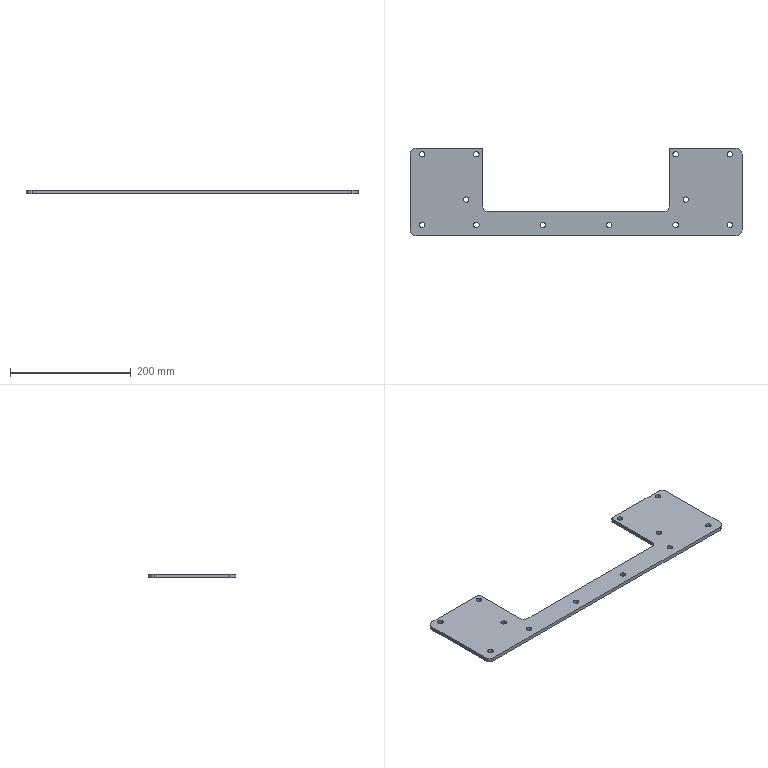Part | SolidWorks | features Fillet 4, HoleWzd 3, MirrorPattern 2, EdgeFlange 1, FlatPattern 1, ICE 1, SMBaseFlange 1, SheetMetal 1 | 1 solid | 42 faces | box 550 x 145 x 6 mm | volume 278339 mm3 | cylinder 32 | plane 10 | commonest cylinder face diameters 9 x24 20 x6 6 x2
STEP:
#1=CARTESIAN_POINT('',(160.5,62.5,0.));
#2=VERTEX_POINT('',#1);
#3=CARTESIAN_POINT('',(169.5,62.5,0.));
#4=VERTEX_POINT('',#3);
#5=CARTESIAN_POINT('',(165.,62.5,0.));
#6=DIRECTION('',(0.,0.,1.));
#7=DIRECTION('',(1.,0.,0.));
#8=AXIS2_PLACEMENT_3D('',#5,#6,#7);
#9=CIRCLE('',#8,4.5);
#10=EDGE_CURVE('',#2,#4,#9,.T.);
#11=ORIENTED_EDGE('',*,*,#10,.T.);
#12=CARTESIAN_POINT('',(169.5,62.5,-6.));
#13=VERTEX_POINT('',#12);
#14=CARTESIAN_POINT('',(169.5,62.5,-6.));
#15=DIRECTION('',(0.,0.,-1.));
#16=VECTOR('',#15,1000.);
#17=LINE('',#14,#16);
#18=EDGE_CURVE('',#4,#13,#17,.T.);
#19=ORIENTED_EDGE('',*,*,#18,.T.);
#20=CARTESIAN_POINT('',(160.5,62.5,-6.));
#21=VERTEX_POINT('',#20);
#22=CARTESIAN_POINT('',(165.,62.5,-6.));
#23=DIRECTION('',(0.,0.,-1.));
#24=DIRECTION('',(-1.,0.,0.));
#25=AXIS2_PLACEMENT_3D('',#22,#23,#24);
#26=CIRCLE('',#25,4.5);
#27=EDGE_CURVE('',#13,#21,#26,.T.);
#28=ORIENTED_EDGE('',*,*,#27,.T.);
#29=CARTESIAN_POINT('',(160.5,62.5,-6.));
#30=DIRECTION('',(0.,0.,-1.));
#31=VECTOR('',#30,1000.);
#32=LINE('',#29,#31);
#33=EDGE_CURVE('',#2,#21,#32,.T.);
#34=ORIENTED_EDGE('',*,*,#33,.F.);
#35=EDGE_LOOP('',(#11,#19,#28,#34));
#36=FACE_OUTER_BOUND('',#35,.T.);
#37=CARTESIAN_POINT('',(165.,62.5,-6.));
#38=DIRECTION('',(0.,0.,-1.));
#39=DIRECTION('',(-1.,0.,0.));
#40=AXIS2_PLACEMENT_3D('',#37,#38,#39);
#41=CYLINDRICAL_SURFACE('',#40,4.5);
#42=ADVANCED_FACE('',(#36),#41,.F.);
#43=CARTESIAN_POINT('',(50.5,-55.,0.));
#44=VERTEX_POINT('',#43);
#45=CARTESIAN_POINT('',(59.5,-55.,0.));
#46=VERTEX_POINT('',#45);
#47=CARTESIAN_POINT('',(55.,-55.,0.));
#48=DIRECTION('',(0.,0.,1.));
#49=DIRECTION('',(1.,0.,0.));
#50=AXIS2_PLACEMENT_3D('',#47,#48,#49);
#51=CIRCLE('',#50,4.5);
#52=EDGE_CURVE('',#44,#46,#51,.T.);
#53=ORIENTED_EDGE('',*,*,#52,.T.);
#54=CARTESIAN_POINT('',(59.5,-55.,-6.));
#55=VERTEX_POINT('',#54);
#56=CARTESIAN_POINT('',(59.5,-55.,-6.));
#57=DIRECTION('',(0.,0.,-1.));
#58=VECTOR('',#57,1000.);
#59=LINE('',#56,#58);
#60=EDGE_CURVE('',#46,#55,#59,.T.);
#61=ORIENTED_EDGE('',*,*,#60,.T.);
#62=CARTESIAN_POINT('',(50.5,-55.,-6.));
#63=VERTEX_POINT('',#62);
#64=CARTESIAN_POINT('',(55.,-55.,-6.));
#65=DIRECTION('',(0.,0.,-1.));
#66=DIRECTION('',(-1.,0.,0.));
#67=AXIS2_PLACEMENT_3D('',#64,#65,#66);
#68=CIRCLE('',#67,4.5);
#69=EDGE_CURVE('',#55,#63,#68,.T.);
#70=ORIENTED_EDGE('',*,*,#69,.T.);
#71=CARTESIAN_POINT('',(50.5,-55.,-6.));
#72=DIRECTION('',(0.,0.,-1.));
#73=VECTOR('',#72,1000.);
#74=LINE('',#71,#73);
#75=EDGE_CURVE('',#44,#63,#74,.T.);
#76=ORIENTED_EDGE('',*,*,#75,.F.);
#77=EDGE_LOOP('',(#53,#61,#70,#76));
#78=FACE_OUTER_BOUND('',#77,.T.);
#79=CARTESIAN_POINT('',(55.,-55.,-6.));
#80=DIRECTION('',(0.,0.,-1.));
#81=DIRECTION('',(-1.,0.,0.));
#82=AXIS2_PLACEMENT_3D('',#79,#80,#81);
#83=CYLINDRICAL_SURFACE('',#82,4.5);
#84=ADVANCED_FACE('',(#78),#83,.F.);
#85=CARTESIAN_POINT('',(-59.5,-55.,0.));
#86=VERTEX_POINT('',#85);
#87=CARTESIAN_POINT('',(-50.5,-55.,0.));
#88=VERTEX_POINT('',#87);
#89=CARTESIAN_POINT('',(-55.,-55.,0.));
#90=DIRECTION('',(0.,0.,1.));
#91=DIRECTION('',(1.,0.,0.));
#92=AXIS2_PLACEMENT_3D('',#89,#90,#91);
#93=CIRCLE('',#92,4.5);
#94=EDGE_CURVE('',#86,#88,#93,.T.);
#95=ORIENTED_EDGE('',*,*,#94,.T.);
#96=CARTESIAN_POINT('',(-50.5,-55.,-6.));
#97=VERTEX_POINT('',#96);
#98=CARTESIAN_POINT('',(-50.5,-55.,-6.));
#99=DIRECTION('',(0.,0.,-1.));
#100=VECTOR('',#99,1000.);
#101=LINE('',#98,#100);
#102=EDGE_CURVE('',#88,#97,#101,.T.);
#103=ORIENTED_EDGE('',*,*,#102,.T.);
#104=CARTESIAN_POINT('',(-59.5,-55.,-6.));
#105=VERTEX_POINT('',#104);
#106=CARTESIAN_POINT('',(-55.,-55.,-6.));
#107=DIRECTION('',(0.,0.,-1.));
#108=DIRECTION('',(-1.,0.,0.));
#109=AXIS2_PLACEMENT_3D('',#106,#107,#108);
#110=CIRCLE('',#109,4.5);
#111=EDGE_CURVE('',#97,#105,#110,.T.);
#112=ORIENTED_EDGE('',*,*,#111,.T.);
#113=CARTESIAN_POINT('',(-59.5,-55.,-6.));
#114=DIRECTION('',(0.,0.,-1.));
#115=VECTOR('',#114,1000.);
#116=LINE('',#113,#115);
#117=EDGE_CURVE('',#86,#105,#116,.T.);
#118=ORIENTED_EDGE('',*,*,#117,.F.);
#119=EDGE_LOOP('',(#95,#103,#112,#118));
#120=FACE_OUTER_BOUND('',#119,.T.);
#121=CARTESIAN_POINT('',(-55.,-55.,-6.));
#122=DIRECTION('',(0.,0.,-1.));
#123=DIRECTION('',(-1.,0.,0.));
#124=AXIS2_PLACEMENT_3D('',#121,#122,#123);
#125=CYLINDRICAL_SURFACE('',#124,4.5);
#126=ADVANCED_FACE('',(#120),#125,.F.);
#127=CARTESIAN_POINT('',(-169.5,-55.,0.));
#128=VERTEX_POINT('',#127);
#129=CARTESIAN_POINT('',(-160.5,-55.,0.));
#130=VERTEX_POINT('',#129);
#131=CARTESIAN_POINT('',(-165.,-55.,0.));
#132=DIRECTION('',(0.,0.,1.));
#133=DIRECTION('',(1.,0.,0.));
#134=AXIS2_PLACEMENT_3D('',#131,#132,#133);
#135=CIRCLE('',#134,4.5);
#136=EDGE_CURVE('',#128,#130,#135,.T.);
#137=ORIENTED_EDGE('',*,*,#136,.T.);
#138=CARTESIAN_POINT('',(-160.5,-55.,-6.));
#139=VERTEX_POINT('',#138);
#140=CARTESIAN_POINT('',(-160.5,-55.,-6.));
#141=DIRECTION('',(0.,0.,-1.));
#142=VECTOR('',#141,1000.);
#143=LINE('',#140,#142);
#144=EDGE_CURVE('',#130,#139,#143,.T.);
#145=ORIENTED_EDGE('',*,*,#144,.T.);
#146=CARTESIAN_POINT('',(-169.5,-55.,-6.));
#147=VERTEX_POINT('',#146);
#148=CARTESIAN_POINT('',(-165.,-55.,-6.));
#149=DIRECTION('',(0.,0.,-1.));
#150=DIRECTION('',(-1.,0.,0.));
#151=AXIS2_PLACEMENT_3D('',#148,#149,#150);
#152=CIRCLE('',#151,4.5);
#153=EDGE_CURVE('',#139,#147,#152,.T.);
#154=ORIENTED_EDGE('',*,*,#153,.T.);
#155=CARTESIAN_POINT('',(-169.5,-55.,-6.));
#156=DIRECTION('',(0.,0.,-1.));
#157=VECTOR('',#156,1000.);
#158=LINE('',#155,#157);
#159=EDGE_CURVE('',#128,#147,#158,.T.);
#160=ORIENTED_EDGE('',*,*,#159,.F.);
#161=EDGE_LOOP('',(#137,#145,#154,#160));
#162=FACE_OUTER_BOUND('',#161,.T.);
#163=CARTESIAN_POINT('',(-165.,-55.,-6.));
#164=DIRECTION('',(0.,0.,-1.));
#165=DIRECTION('',(-1.,0.,0.));
#166=AXIS2_PLACEMENT_3D('',#163,#164,#165);
#167=CYLINDRICAL_SURFACE('',#166,4.5);
#168=ADVANCED_FACE('',(#162),#167,.F.);
#169=CARTESIAN_POINT('',(-169.5,62.5,0.));
#170=VERTEX_POINT('',#169);
#171=CARTESIAN_POINT('',(-160.5,62.5,0.));
#172=VERTEX_POINT('',#171);
#173=CARTESIAN_POINT('',(-165.,62.5,0.));
#174=DIRECTION('',(0.,0.,1.));
#175=DIRECTION('',(1.,0.,0.));
#176=AXIS2_PLACEMENT_3D('',#173,#174,#175);
#177=CIRCLE('',#176,4.5);
#178=EDGE_CURVE('',#170,#172,#177,.T.);
#179=ORIENTED_EDGE('',*,*,#178,.T.);
#180=CARTESIAN_POINT('',(-160.5,62.5,-6.));
#181=VERTEX_POINT('',#180);
#182=CARTESIAN_POINT('',(-160.5,62.5,-6.));
#183=DIRECTION('',(0.,0.,-1.));
#184=VECTOR('',#183,1000.);
#185=LINE('',#182,#184);
#186=EDGE_CURVE('',#172,#181,#185,.T.);
#187=ORIENTED_EDGE('',*,*,#186,.T.);
#188=CARTESIAN_POINT('',(-169.5,62.5,-6.));
#189=VERTEX_POINT('',#188);
#190=CARTESIAN_POINT('',(-165.,62.5,-6.));
#191=DIRECTION('',(0.,0.,-1.));
#192=DIRECTION('',(-1.,0.,0.));
#193=AXIS2_PLACEMENT_3D('',#190,#191,#192);
#194=CIRCLE('',#193,4.5);
#195=EDGE_CURVE('',#181,#189,#194,.T.);
#196=ORIENTED_EDGE('',*,*,#195,.T.);
#197=CARTESIAN_POINT('',(-169.5,62.5,-6.));
#198=DIRECTION('',(0.,0.,-1.));
#199=VECTOR('',#198,1000.);
#200=LINE('',#197,#199);
#201=EDGE_CURVE('',#170,#189,#200,.T.);
#202=ORIENTED_EDGE('',*,*,#201,.F.);
#203=EDGE_LOOP('',(#179,#187,#196,#202));
#204=FACE_OUTER_BOUND('',#203,.T.);
#205=CARTESIAN_POINT('',(-165.,62.5,-6.));
#206=DIRECTION('',(0.,0.,-1.));
#207=DIRECTION('',(-1.,0.,0.));
#208=AXIS2_PLACEMENT_3D('',#205,#206,#207);
#209=CYLINDRICAL_SURFACE('',#208,4.5);
#210=ADVANCED_FACE('',(#204),#209,.F.);
#211=CARTESIAN_POINT('',(160.5,-55.,0.));
#212=VERTEX_POINT('',#211);
#213=CARTESIAN_POINT('',(169.5,-55.,0.));
#214=VERTEX_POINT('',#213);
#215=CARTESIAN_POINT('',(165.,-55.,0.));
#216=DIRECTION('',(0.,0.,1.));
#217=DIRECTION('',(1.,0.,0.));
#218=AXIS2_PLACEMENT_3D('',#215,#216,#217);
#219=CIRCLE('',#218,4.5);
#220=EDGE_CURVE('',#212,#214,#219,.T.);
#221=ORIENTED_EDGE('',*,*,#220,.T.);
#222=CARTESIAN_POINT('',(169.5,-55.,-6.));
#223=VERTEX_POINT('',#222);
#224=CARTESIAN_POINT('',(169.5,-55.,-6.));
#225=DIRECTION('',(0.,0.,-1.));
#226=VECTOR('',#225,1000.);
#227=LINE('',#224,#226);
#228=EDGE_CURVE('',#214,#223,#227,.T.);
#229=ORIENTED_EDGE('',*,*,#228,.T.);
#230=CARTESIAN_POINT('',(160.5,-55.,-6.));
#231=VERTEX_POINT('',#230);
#232=CARTESIAN_POINT('',(165.,-55.,-6.));
#233=DIRECTION('',(0.,0.,-1.));
#234=DIRECTION('',(-1.,0.,0.));
#235=AXIS2_PLACEMENT_3D('',#232,#233,#234);
#236=CIRCLE('',#235,4.5);
#237=EDGE_CURVE('',#223,#231,#236,.T.);
#238=ORIENTED_EDGE('',*,*,#237,.T.);
#239=CARTESIAN_POINT('',(160.5,-55.,-6.));
#240=DIRECTION('',(0.,0.,-1.));
#241=VECTOR('',#240,1000.);
#242=LINE('',#239,#241);
#243=EDGE_CURVE('',#212,#231,#242,.T.);
#244=ORIENTED_EDGE('',*,*,#243,.F.);
#245=EDGE_LOOP('',(#221,#229,#238,#244));
#246=FACE_OUTER_BOUND('',#245,.T.);
#247=CARTESIAN_POINT('',(165.,-55.,-6.));
#248=DIRECTION('',(0.,0.,-1.));
#249=DIRECTION('',(-1.,0.,0.));
#250=AXIS2_PLACEMENT_3D('',#247,#248,#249);
#251=CYLINDRICAL_SURFACE('',#250,4.5);
#252=ADVANCED_FACE('',(#246),#251,.F.);
#253=CARTESIAN_POINT('',(-259.5,-55.,0.));
#254=VERTEX_POINT('',#253);
#255=CARTESIAN_POINT('',(-250.5,-55.,0.));
#256=VERTEX_POINT('',#255);
#257=CARTESIAN_POINT('',(-255.,-55.,0.));
#258=DIRECTION('',(0.,0.,1.));
#259=DIRECTION('',(1.,0.,0.));
#260=AXIS2_PLACEMENT_3D('',#257,#258,#259);
#261=CIRCLE('',#260,4.5);
#262=EDGE_CURVE('',#254,#256,#261,.T.);
#263=ORIENTED_EDGE('',*,*,#262,.T.);
#264=CARTESIAN_POINT('',(-250.5,-55.,-6.));
#265=VERTEX_POINT('',#264);
#266=CARTESIAN_POINT('',(-250.5,-55.,-6.));
#267=DIRECTION('',(0.,0.,-1.));
#268=VECTOR('',#267,1000.);
#269=LINE('',#266,#268);
#270=EDGE_CURVE('',#256,#265,#269,.T.);
#271=ORIENTED_EDGE('',*,*,#270,.T.);
#272=CARTESIAN_POINT('',(-259.5,-55.,-6.));
#273=VERTEX_POINT('',#272);
#274=CARTESIAN_POINT('',(-255.,-55.,-6.));
#275=DIRECTION('',(0.,0.,-1.));
#276=DIRECTION('',(-1.,0.,0.));
#277=AXIS2_PLACEMENT_3D('',#274,#275,#276);
#278=CIRCLE('',#277,4.5);
#279=EDGE_CURVE('',#265,#273,#278,.T.);
#280=ORIENTED_EDGE('',*,*,#279,.T.);
#281=CARTESIAN_POINT('',(-259.5,-55.,-6.));
#282=DIRECTION('',(0.,0.,-1.));
#283=VECTOR('',#282,1000.);
#284=LINE('',#281,#283);
#285=EDGE_CURVE('',#254,#273,#284,.T.);
#286=ORIENTED_EDGE('',*,*,#285,.F.);
#287=EDGE_LOOP('',(#263,#271,#280,#286));
#288=FACE_OUTER_BOUND('',#287,.T.);
#289=CARTESIAN_POINT('',(-255.,-55.,-6.));
#290=DIRECTION('',(0.,0.,-1.));
#291=DIRECTION('',(-1.,0.,0.));
#292=AXIS2_PLACEMENT_3D('',#289,#290,#291);
#293=CYLINDRICAL_SURFACE('',#292,4.5);
#294=ADVANCED_FACE('',(#288),#293,.F.);
#295=CARTESIAN_POINT('',(250.5,-55.,0.));
#296=VERTEX_POINT('',#295);
#297=CARTESIAN_POINT('',(259.5,-55.,0.));
#298=VERTEX_POINT('',#297);
#299=CARTESIAN_POINT('',(255.,-55.,0.));
#300=DIRECTION('',(0.,0.,1.));
#301=DIRECTION('',(1.,0.,0.));
#302=AXIS2_PLACEMENT_3D('',#299,#300,#301);
#303=CIRCLE('',#302,4.5);
#304=EDGE_CURVE('',#296,#298,#303,.T.);
#305=ORIENTED_EDGE('',*,*,#304,.T.);
#306=CARTESIAN_POINT('',(259.5,-55.,-6.));
#307=VERTEX_POINT('',#306);
#308=CARTESIAN_POINT('',(259.5,-55.,-6.));
#309=DIRECTION('',(0.,0.,-1.));
#310=VECTOR('',#309,1000.);
#311=LINE('',#308,#310);
#312=EDGE_CURVE('',#298,#307,#311,.T.);
#313=ORIENTED_EDGE('',*,*,#312,.T.);
#314=CARTESIAN_POINT('',(250.5,-55.,-6.));
#315=VERTEX_POINT('',#314);
#316=CARTESIAN_POINT('',(255.,-55.,-6.));
#317=DIRECTION('',(0.,0.,-1.));
#318=DIRECTION('',(-1.,0.,0.));
#319=AXIS2_PLACEMENT_3D('',#316,#317,#318);
#320=CIRCLE('',#319,4.5);
#321=EDGE_CURVE('',#307,#315,#320,.T.);
#322=ORIENTED_EDGE('',*,*,#321,.T.);
#323=CARTESIAN_POINT('',(250.5,-55.,-6.));
#324=DIRECTION('',(0.,0.,-1.));
#325=VECTOR('',#324,1000.);
#326=LINE('',#323,#325);
#327=EDGE_CURVE('',#296,#315,#326,.T.);
#328=ORIENTED_EDGE('',*,*,#327,.F.);
#329=EDGE_LOOP('',(#305,#313,#322,#328));
#330=FACE_OUTER_BOUND('',#329,.T.);
#331=CARTESIAN_POINT('',(255.,-55.,-6.));
#332=DIRECTION('',(0.,0.,-1.));
#333=DIRECTION('',(-1.,0.,0.));
#334=AXIS2_PLACEMENT_3D('',#331,#332,#333);
#335=CYLINDRICAL_SURFACE('',#334,4.5);
#336=ADVANCED_FACE('',(#330),#335,.F.);
#337=CARTESIAN_POINT('',(250.5,62.5,0.));
#338=VERTEX_POINT('',#337);
#339=CARTESIAN_POINT('',(259.5,62.5,0.));
#340=VERTEX_POINT('',#339);
#341=CARTESIAN_POINT('',(255.,62.5,0.));
#342=DIRECTION('',(0.,0.,1.));
#343=DIRECTION('',(1.,0.,0.));
#344=AXIS2_PLACEMENT_3D('',#341,#342,#343);
#345=CIRCLE('',#344,4.5);
#346=EDGE_CURVE('',#338,#340,#345,.T.);
#347=ORIENTED_EDGE('',*,*,#346,.T.);
#348=CARTESIAN_POINT('',(259.5,62.5,-6.));
#349=VERTEX_POINT('',#348);
#350=CARTESIAN_POINT('',(259.5,62.5,-6.));
#351=DIRECTION('',(0.,0.,-1.));
#352=VECTOR('',#351,1000.);
#353=LINE('',#350,#352);
#354=EDGE_CURVE('',#340,#349,#353,.T.);
#355=ORIENTED_EDGE('',*,*,#354,.T.);
#356=CARTESIAN_POINT('',(250.5,62.5,-6.));
#357=VERTEX_POINT('',#356);
#358=CARTESIAN_POINT('',(255.,62.5,-6.));
#359=DIRECTION('',(0.,0.,-1.));
#360=DIRECTION('',(-1.,0.,0.));
#361=AXIS2_PLACEMENT_3D('',#358,#359,#360);
#362=CIRCLE('',#361,4.5);
#363=EDGE_CURVE('',#349,#357,#362,.T.);
#364=ORIENTED_EDGE('',*,*,#363,.T.);
#365=CARTESIAN_POINT('',(250.5,62.5,-6.));
#366=DIRECTION('',(0.,0.,-1.));
#367=VECTOR('',#366,1000.);
#368=LINE('',#365,#367);
#369=EDGE_CURVE('',#338,#357,#368,.T.);
#370=ORIENTED_EDGE('',*,*,#369,.F.);
#371=EDGE_LOOP('',(#347,#355,#364,#370));
#372=FACE_OUTER_BOUND('',#371,.T.);
#373=CARTESIAN_POINT('',(255.,62.5,-6.));
#374=DIRECTION('',(0.,0.,-1.));
#375=DIRECTION('',(-1.,0.,0.));
#376=AXIS2_PLACEMENT_3D('',#373,#374,#375);
#377=CYLINDRICAL_SURFACE('',#376,4.5);
#378=ADVANCED_FACE('',(#372),#377,.F.);
#379=CARTESIAN_POINT('',(-259.5,62.5,0.));
#380=VERTEX_POINT('',#379);
#381=CARTESIAN_POINT('',(-250.5,62.5,0.));
#382=VERTEX_POINT('',#381);
#383=CARTESIAN_POINT('',(-255.,62.5,0.));
#384=DIRECTION('',(0.,0.,1.));
#385=DIRECTION('',(1.,0.,0.));
#386=AXIS2_PLACEMENT_3D('',#383,#384,#385);
#387=CIRCLE('',#386,4.5);
#388=EDGE_CURVE('',#380,#382,#387,.T.);
#389=ORIENTED_EDGE('',*,*,#388,.T.);
#390=CARTESIAN_POINT('',(-250.5,62.5,-6.));
#391=VERTEX_POINT('',#390);
#392=CARTESIAN_POINT('',(-250.5,62.5,-6.));
#393=DIRECTION('',(0.,0.,-1.));
#394=VECTOR('',#393,1000.);
#395=LINE('',#392,#394);
#396=EDGE_CURVE('',#382,#391,#395,.T.);
#397=ORIENTED_EDGE('',*,*,#396,.T.);
#398=CARTESIAN_POINT('',(-259.5,62.5,-6.));
#399=VERTEX_POINT('',#398);
#400=CARTESIAN_POINT('',(-255.,62.5,-6.));
#401=DIRECTION('',(0.,0.,-1.));
#402=DIRECTION('',(-1.,0.,0.));
#403=AXIS2_PLACEMENT_3D('',#400,#401,#402);
#404=CIRCLE('',#403,4.5);
#405=EDGE_CURVE('',#391,#399,#404,.T.);
#406=ORIENTED_EDGE('',*,*,#405,.T.);
#407=CARTESIAN_POINT('',(-259.5,62.5,-6.));
#408=DIRECTION('',(0.,0.,-1.));
#409=VECTOR('',#408,1000.);
#410=LINE('',#407,#409);
#411=EDGE_CURVE('',#380,#399,#410,.T.);
#412=ORIENTED_EDGE('',*,*,#411,.F.);
#413=EDGE_LOOP('',(#389,#397,#406,#412));
#414=FACE_OUTER_BOUND('',#413,.T.);
#415=CARTESIAN_POINT('',(-255.,62.5,-6.));
#416=DIRECTION('',(0.,0.,-1.));
#417=DIRECTION('',(-1.,0.,0.));
#418=AXIS2_PLACEMENT_3D('',#415,#416,#417);
#419=CYLINDRICAL_SURFACE('',#418,4.5);
#420=ADVANCED_FACE('',(#414),#419,.F.);
#421=CARTESIAN_POINT('',(177.5,-12.5,-6.));
#422=VERTEX_POINT('',#421);
#423=CARTESIAN_POINT('',(186.5,-12.5,-6.));
#424=VERTEX_POINT('',#423);
#425=CARTESIAN_POINT('',(182.,-12.5,-6.));
#426=DIRECTION('',(0.,0.,1.));
#427=DIRECTION('',(1.,0.,0.));
#428=AXIS2_PLACEMENT_3D('',#425,#426,#427);
#429=CIRCLE('',#428,4.5);
#430=EDGE_CURVE('',#422,#424,#429,.T.);
#431=ORIENTED_EDGE('',*,*,#430,.F.);
#432=CARTESIAN_POINT('',(177.5,-12.5,0.));
#433=VERTEX_POINT('',#432);
#434=CARTESIAN_POINT('',(177.5,-12.5,0.));
#435=DIRECTION('',(0.,0.,1.));
#436=VECTOR('',#435,1000.);
#437=LINE('',#434,#436);
#438=EDGE_CURVE('',#422,#433,#437,.T.);
#439=ORIENTED_EDGE('',*,*,#438,.T.);
#440=CARTESIAN_POINT('',(186.5,-12.5,0.));
#441=VERTEX_POINT('',#440);
#442=CARTESIAN_POINT('',(182.,-12.5,0.));
#443=DIRECTION('',(0.,0.,1.));
#444=DIRECTION('',(1.,0.,0.));
#445=AXIS2_PLACEMENT_3D('',#442,#443,#444);
#446=CIRCLE('',#445,4.5);
#447=EDGE_CURVE('',#433,#441,#446,.T.);
#448=ORIENTED_EDGE('',*,*,#447,.T.);
#449=CARTESIAN_POINT('',(186.5,-12.5,0.));
#450=DIRECTION('',(0.,0.,1.));
#451=VECTOR('',#450,1000.);
#452=LINE('',#449,#451);
#453=EDGE_CURVE('',#424,#441,#452,.T.);
#454=ORIENTED_EDGE('',*,*,#453,.F.);
#455=EDGE_LOOP('',(#431,#439,#448,#454));
#456=FACE_OUTER_BOUND('',#455,.T.);
#457=CARTESIAN_POINT('',(182.,-12.5,0.));
#458=DIRECTION('',(0.,0.,1.));
#459=DIRECTION('',(1.,0.,0.));
#460=AXIS2_PLACEMENT_3D('',#457,#458,#459);
#461=CYLINDRICAL_SURFACE('',#460,4.5);
#462=ADVANCED_FACE('',(#456),#461,.F.);
#463=CARTESIAN_POINT('',(-186.5,-12.5,-6.));
#464=VERTEX_POINT('',#463);
#465=CARTESIAN_POINT('',(-177.5,-12.5,-6.));
#466=VERTEX_POINT('',#465);
#467=CARTESIAN_POINT('',(-182.,-12.5,-6.));
#468=DIRECTION('',(0.,0.,1.));
#469=DIRECTION('',(1.,0.,0.));
#470=AXIS2_PLACEMENT_3D('',#467,#468,#469);
#471=CIRCLE('',#470,4.5);
#472=EDGE_CURVE('',#464,#466,#471,.T.);
#473=ORIENTED_EDGE('',*,*,#472,.F.);
#474=CARTESIAN_POINT('',(-186.5,-12.5,0.));
#475=VERTEX_POINT('',#474);
#476=CARTESIAN_POINT('',(-186.5,-12.5,0.));
#477=DIRECTION('',(0.,0.,1.));
#478=VECTOR('',#477,1000.);
#479=LINE('',#476,#478);
#480=EDGE_CURVE('',#464,#475,#479,.T.);
#481=ORIENTED_EDGE('',*,*,#480,.T.);
#482=CARTESIAN_POINT('',(-177.5,-12.5,0.));
#483=VERTEX_POINT('',#482);
#484=CARTESIAN_POINT('',(-182.,-12.5,0.));
#485=DIRECTION('',(0.,0.,1.));
#486=DIRECTION('',(1.,0.,0.));
#487=AXIS2_PLACEMENT_3D('',#484,#485,#486);
#488=CIRCLE('',#487,4.5);
#489=EDGE_CURVE('',#475,#483,#488,.T.);
#490=ORIENTED_EDGE('',*,*,#489,.T.);
#491=CARTESIAN_POINT('',(-177.5,-12.5,0.));
#492=DIRECTION('',(0.,0.,1.));
#493=VECTOR('',#492,1000.);
#494=LINE('',#491,#493);
#495=EDGE_CURVE('',#466,#483,#494,.T.);
#496=ORIENTED_EDGE('',*,*,#495,.F.);
#497=EDGE_LOOP('',(#473,#481,#490,#496));
#498=FACE_OUTER_BOUND('',#497,.T.);
#499=CARTESIAN_POINT('',(-182.,-12.5,0.));
#500=DIRECTION('',(0.,0.,1.));
#501=DIRECTION('',(1.,0.,0.));
#502=AXIS2_PLACEMENT_3D('',#499,#500,#501);
#503=CYLINDRICAL_SURFACE('',#502,4.5);
#504=ADVANCED_FACE('',(#498),#503,.F.);
#505=CARTESIAN_POINT('',(-165.,62.5,-6.));
#506=DIRECTION('',(0.,0.,-1.));
#507=DIRECTION('',(-1.,0.,0.));
#508=AXIS2_PLACEMENT_3D('',#505,#506,#507);
#509=CIRCLE('',#508,4.5);
#510=EDGE_CURVE('',#189,#181,#509,.T.);
#511=ORIENTED_EDGE('',*,*,#510,.F.);
#512=ORIENTED_EDGE('',*,*,#195,.F.);
#513=EDGE_LOOP('',(#511,#512));
#514=FACE_BOUND('',#513,.T.);
#515=CARTESIAN_POINT('',(165.,-55.,-6.));
#516=DIRECTION('',(0.,0.,-1.));
#517=DIRECTION('',(-1.,0.,0.));
#518=AXIS2_PLACEMENT_3D('',#515,#516,#517);
#519=CIRCLE('',#518,4.5);
#520=EDGE_CURVE('',#231,#223,#519,.T.);
#521=ORIENTED_EDGE('',*,*,#520,.F.);
#522=ORIENTED_EDGE('',*,*,#237,.F.);
#523=EDGE_LOOP('',(#521,#522));
#524=FACE_BOUND('',#523,.T.);
#525=CARTESIAN_POINT('',(-255.,-55.,-6.));
#526=DIRECTION('',(0.,0.,-1.));
#527=DIRECTION('',(-1.,0.,0.));
#528=AXIS2_PLACEMENT_3D('',#525,#526,#527);
#529=CIRCLE('',#528,4.5);
#530=EDGE_CURVE('',#273,#265,#529,.T.);
#531=ORIENTED_EDGE('',*,*,#530,.F.);
#532=ORIENTED_EDGE('',*,*,#279,.F.);
#533=EDGE_LOOP('',(#531,#532));
#534=FACE_BOUND('',#533,.T.);
#535=CARTESIAN_POINT('',(255.,-55.,-6.));
#536=DIRECTION('',(0.,0.,-1.));
#537=DIRECTION('',(-1.,0.,0.));
#538=AXIS2_PLACEMENT_3D('',#535,#536,#537);
#539=CIRCLE('',#538,4.5);
#540=EDGE_CURVE('',#315,#307,#539,.T.);
#541=ORIENTED_EDGE('',*,*,#540,.F.);
#542=ORIENTED_EDGE('',*,*,#321,.F.);
#543=EDGE_LOOP('',(#541,#542));
#544=FACE_BOUND('',#543,.T.);
#545=CARTESIAN_POINT('',(255.,62.5,-6.));
#546=DIRECTION('',(0.,0.,-1.));
#547=DIRECTION('',(-1.,0.,0.));
#548=AXIS2_PLACEMENT_3D('',#545,#546,#547);
#549=CIRCLE('',#548,4.5);
#550=EDGE_CURVE('',#357,#349,#549,.T.);
#551=ORIENTED_EDGE('',*,*,#550,.F.);
#552=ORIENTED_EDGE('',*,*,#363,.F.);
#553=EDGE_LOOP('',(#551,#552));
#554=FACE_BOUND('',#553,.T.);
#555=CARTESIAN_POINT('',(-255.,62.5,-6.));
#556=DIRECTION('',(0.,0.,-1.));
#557=DIRECTION('',(-1.,0.,0.));
#558=AXIS2_PLACEMENT_3D('',#555,#556,#557);
#559=CIRCLE('',#558,4.5);
#560=EDGE_CURVE('',#399,#391,#559,.T.);
#561=ORIENTED_EDGE('',*,*,#560,.F.);
#562=ORIENTED_EDGE('',*,*,#405,.F.);
#563=EDGE_LOOP('',(#561,#562));
#564=FACE_BOUND('',#563,.T.);
#565=CARTESIAN_POINT('',(182.,-12.5,-6.));
#566=DIRECTION('',(0.,0.,1.));
#567=DIRECTION('',(1.,0.,0.));
#568=AXIS2_PLACEMENT_3D('',#565,#566,#567);
#569=CIRCLE('',#568,4.5);
#570=EDGE_CURVE('',#424,#422,#569,.T.);
#571=ORIENTED_EDGE('',*,*,#570,.T.);
#572=ORIENTED_EDGE('',*,*,#430,.T.);
#573=EDGE_LOOP('',(#571,#572));
#574=FACE_BOUND('',#573,.T.);
#575=CARTESIAN_POINT('',(-182.,-12.5,-6.));
#576=DIRECTION('',(0.,0.,1.));
#577=DIRECTION('',(1.,0.,0.));
#578=AXIS2_PLACEMENT_3D('',#575,#576,#577);
#579=CIRCLE('',#578,4.5);
#580=EDGE_CURVE('',#466,#464,#579,.T.);
#581=ORIENTED_EDGE('',*,*,#580,.T.);
#582=ORIENTED_EDGE('',*,*,#472,.T.);
#583=EDGE_LOOP('',(#581,#582));
#584=FACE_BOUND('',#583,.T.);
#585=CARTESIAN_POINT('',(155.,-22.5,-6.));
#586=VERTEX_POINT('',#585);
#587=CARTESIAN_POINT('',(155.,69.5,-6.));
#588=VERTEX_POINT('',#587);
#589=CARTESIAN_POINT('',(155.,72.5,-6.));
#590=DIRECTION('',(0.,1.,0.));
#591=VECTOR('',#590,1000.);
#592=LINE('',#589,#591);
#593=EDGE_CURVE('',#586,#588,#592,.T.);
#594=ORIENTED_EDGE('',*,*,#593,.T.);
#595=CARTESIAN_POINT('',(158.,72.5,-6.));
#596=VERTEX_POINT('',#595);
#597=CARTESIAN_POINT('',(158.,69.5,-6.));
#598=DIRECTION('',(0.,0.,-1.));
#599=DIRECTION('',(1.,0.,0.));
#600=AXIS2_PLACEMENT_3D('',#597,#598,#599);
#601=CIRCLE('',#600,3.);
#602=EDGE_CURVE('',#588,#596,#601,.T.);
#603=ORIENTED_EDGE('',*,*,#602,.T.);
#604=CARTESIAN_POINT('',(265.,72.5,-6.));
#605=VERTEX_POINT('',#604);
#606=CARTESIAN_POINT('',(-275.,72.5,-6.));
#607=DIRECTION('',(-1.,0.,0.));
#608=VECTOR('',#607,1000.);
#609=LINE('',#606,#608);
#610=EDGE_CURVE('',#605,#596,#609,.T.);
#611=ORIENTED_EDGE('',*,*,#610,.F.);
#612=CARTESIAN_POINT('',(275.,62.5,-6.));
#613=VERTEX_POINT('',#612);
#614=CARTESIAN_POINT('',(265.,62.5,-6.));
#615=DIRECTION('',(0.,0.,-1.));
#616=DIRECTION('',(1.,0.,0.));
#617=AXIS2_PLACEMENT_3D('',#614,#615,#616);
#618=CIRCLE('',#617,10.);
#619=EDGE_CURVE('',#605,#613,#618,.T.);
#620=ORIENTED_EDGE('',*,*,#619,.T.);
#621=CARTESIAN_POINT('',(275.,-62.5,-6.));
#622=VERTEX_POINT('',#621);
#623=CARTESIAN_POINT('',(275.,72.5,-6.));
#624=DIRECTION('',(0.,1.,0.));
#625=VECTOR('',#624,1000.);
#626=LINE('',#623,#625);
#627=EDGE_CURVE('',#622,#613,#626,.T.);
#628=ORIENTED_EDGE('',*,*,#627,.F.);
#629=CARTESIAN_POINT('',(265.,-72.5,-6.));
#630=VERTEX_POINT('',#629);
#631=CARTESIAN_POINT('',(265.,-62.5,-6.));
#632=DIRECTION('',(0.,0.,-1.));
#633=DIRECTION('',(1.,0.,0.));
#634=AXIS2_PLACEMENT_3D('',#631,#632,#633);
#635=CIRCLE('',#634,10.);
#636=EDGE_CURVE('',#622,#630,#635,.T.);
#637=ORIENTED_EDGE('',*,*,#636,.T.);
#638=CARTESIAN_POINT('',(-265.,-72.5,-6.));
#639=VERTEX_POINT('',#638);
#640=CARTESIAN_POINT('',(-275.,-72.5,-6.));
#641=DIRECTION('',(1.,0.,0.));
#642=VECTOR('',#641,1000.);
#643=LINE('',#640,#642);
#644=EDGE_CURVE('',#639,#630,#643,.T.);
#645=ORIENTED_EDGE('',*,*,#644,.F.);
#646=CARTESIAN_POINT('',(-275.,-62.5,-6.));
#647=VERTEX_POINT('',#646);
#648=CARTESIAN_POINT('',(-265.,-62.5,-6.));
#649=DIRECTION('',(0.,0.,-1.));
#650=DIRECTION('',(1.,0.,0.));
#651=AXIS2_PLACEMENT_3D('',#648,#649,#650);
#652=CIRCLE('',#651,10.);
#653=EDGE_CURVE('',#639,#647,#652,.T.);
#654=ORIENTED_EDGE('',*,*,#653,.T.);
#655=CARTESIAN_POINT('',(-275.,62.5,-6.));
#656=VERTEX_POINT('',#655);
#657=CARTESIAN_POINT('',(-275.,72.5,-6.));
#658=DIRECTION('',(0.,-1.,0.));
#659=VECTOR('',#658,1000.);
#660=LINE('',#657,#659);
#661=EDGE_CURVE('',#656,#647,#660,.T.);
#662=ORIENTED_EDGE('',*,*,#661,.F.);
#663=CARTESIAN_POINT('',(-265.,72.5,-6.));
#664=VERTEX_POINT('',#663);
#665=CARTESIAN_POINT('',(-265.,62.5,-6.));
#666=DIRECTION('',(0.,0.,-1.));
#667=DIRECTION('',(1.,0.,0.));
#668=AXIS2_PLACEMENT_3D('',#665,#666,#667);
#669=CIRCLE('',#668,10.);
#670=EDGE_CURVE('',#656,#664,#669,.T.);
#671=ORIENTED_EDGE('',*,*,#670,.T.);
#672=CARTESIAN_POINT('',(-158.,72.5,-6.));
#673=VERTEX_POINT('',#672);
#674=CARTESIAN_POINT('',(-275.,72.5,-6.));
#675=DIRECTION('',(-1.,0.,0.));
#676=VECTOR('',#675,1000.);
#677=LINE('',#674,#676);
#678=EDGE_CURVE('',#673,#664,#677,.T.);
#679=ORIENTED_EDGE('',*,*,#678,.F.);
#680=CARTESIAN_POINT('',(-155.,69.5,-6.));
#681=VERTEX_POINT('',#680);
#682=CARTESIAN_POINT('',(-158.,69.5,-6.));
#683=DIRECTION('',(0.,0.,-1.));
#684=DIRECTION('',(1.,0.,0.));
#685=AXIS2_PLACEMENT_3D('',#682,#683,#684);
#686=CIRCLE('',#685,3.);
#687=EDGE_CURVE('',#673,#681,#686,.T.);
#688=ORIENTED_EDGE('',*,*,#687,.T.);
#689=CARTESIAN_POINT('',(-155.,-22.5,-6.));
#690=VERTEX_POINT('',#689);
#691=CARTESIAN_POINT('',(-155.,72.5,-6.));
#692=DIRECTION('',(0.,-1.,0.));
#693=VECTOR('',#692,1000.);
#694=LINE('',#691,#693);
#695=EDGE_CURVE('',#681,#690,#694,.T.);
#696=ORIENTED_EDGE('',*,*,#695,.T.);
#697=CARTESIAN_POINT('',(-145.,-32.5,-6.));
#698=VERTEX_POINT('',#697);
#699=CARTESIAN_POINT('',(-145.,-22.5,-6.));
#700=DIRECTION('',(0.,0.,1.));
#701=DIRECTION('',(1.,0.,0.));
#702=AXIS2_PLACEMENT_3D('',#699,#700,#701);
#703=CIRCLE('',#702,10.);
#704=EDGE_CURVE('',#690,#698,#703,.T.);
#705=ORIENTED_EDGE('',*,*,#704,.T.);
#706=CARTESIAN_POINT('',(145.,-32.5,-6.));
#707=VERTEX_POINT('',#706);
#708=CARTESIAN_POINT('',(-155.,-32.5,-6.));
#709=DIRECTION('',(1.,0.,0.));
#710=VECTOR('',#709,1000.);
#711=LINE('',#708,#710);
#712=EDGE_CURVE('',#698,#707,#711,.T.);
#713=ORIENTED_EDGE('',*,*,#712,.T.);
#714=CARTESIAN_POINT('',(145.,-22.5,-6.));
#715=DIRECTION('',(0.,0.,1.));
#716=DIRECTION('',(1.,0.,0.));
#717=AXIS2_PLACEMENT_3D('',#714,#715,#716);
#718=CIRCLE('',#717,10.);
#719=EDGE_CURVE('',#707,#586,#718,.T.);
#720=ORIENTED_EDGE('',*,*,#719,.T.);
#721=EDGE_LOOP('',(#594,#603,#611,#620,#628,#637,#645,#654,#662,#671,#679,#688,#696,#705,#713,#720));
#722=FACE_OUTER_BOUND('',#721,.T.);
#723=CARTESIAN_POINT('',(-165.,-55.,-6.));
#724=DIRECTION('',(0.,0.,-1.));
#725=DIRECTION('',(-1.,0.,0.));
#726=AXIS2_PLACEMENT_3D('',#723,#724,#725);
#727=CIRCLE('',#726,4.5);
#728=EDGE_CURVE('',#147,#139,#727,.T.);
#729=ORIENTED_EDGE('',*,*,#728,.F.);
#730=ORIENTED_EDGE('',*,*,#153,.F.);
#731=EDGE_LOOP('',(#729,#730));
#732=FACE_BOUND('',#731,.T.);
#733=CARTESIAN_POINT('',(-55.,-55.,-6.));
#734=DIRECTION('',(0.,0.,-1.));
#735=DIRECTION('',(-1.,0.,0.));
#736=AXIS2_PLACEMENT_3D('',#733,#734,#735);
#737=CIRCLE('',#736,4.5);
#738=EDGE_CURVE('',#105,#97,#737,.T.);
#739=ORIENTED_EDGE('',*,*,#738,.F.);
#740=ORIENTED_EDGE('',*,*,#111,.F.);
#741=EDGE_LOOP('',(#739,#740));
#742=FACE_BOUND('',#741,.T.);
#743=CARTESIAN_POINT('',(55.,-55.,-6.));
#744=DIRECTION('',(0.,0.,-1.));
#745=DIRECTION('',(-1.,0.,0.));
#746=AXIS2_PLACEMENT_3D('',#743,#744,#745);
#747=CIRCLE('',#746,4.5);
#748=EDGE_CURVE('',#63,#55,#747,.T.);
#749=ORIENTED_EDGE('',*,*,#748,.F.);
#750=ORIENTED_EDGE('',*,*,#69,.F.);
#751=EDGE_LOOP('',(#749,#750));
#752=FACE_BOUND('',#751,.T.);
#753=CARTESIAN_POINT('',(165.,62.5,-6.));
#754=DIRECTION('',(0.,0.,-1.));
#755=DIRECTION('',(-1.,0.,0.));
#756=AXIS2_PLACEMENT_3D('',#753,#754,#755);
#757=CIRCLE('',#756,4.5);
#758=EDGE_CURVE('',#21,#13,#757,.T.);
#759=ORIENTED_EDGE('',*,*,#758,.F.);
#760=ORIENTED_EDGE('',*,*,#27,.F.);
#761=EDGE_LOOP('',(#759,#760));
#762=FACE_BOUND('',#761,.T.);
#763=CARTESIAN_POINT('',(0.,0.,-6.));
#764=DIRECTION('',(0.,0.,1.));
#765=DIRECTION('',(1.,0.,0.));
#766=AXIS2_PLACEMENT_3D('',#763,#764,#765);
#767=PLANE('',#766);
#768=ADVANCED_FACE('',(#514,#524,#534,#544,#554,#564,#574,#584,#722,#732,#742,#752,#762),#767,.F.);
#769=CARTESIAN_POINT('',(-158.,72.5,0.));
#770=VERTEX_POINT('',#769);
#771=CARTESIAN_POINT('',(-265.,72.5,0.));
#772=VERTEX_POINT('',#771);
#773=CARTESIAN_POINT('',(-275.,72.5,0.));
#774=DIRECTION('',(-1.,0.,0.));
#775=VECTOR('',#774,1000.);
#776=LINE('',#773,#775);
#777=EDGE_CURVE('',#770,#772,#776,.T.);
#778=ORIENTED_EDGE('',*,*,#777,.F.);
#779=CARTESIAN_POINT('',(-158.,72.5,-6.));
#780=DIRECTION('',(0.,0.,-1.));
#781=VECTOR('',#780,1000.);
#782=LINE('',#779,#781);
#783=EDGE_CURVE('',#770,#673,#782,.T.);
#784=ORIENTED_EDGE('',*,*,#783,.T.);
#785=ORIENTED_EDGE('',*,*,#678,.T.);
#786=CARTESIAN_POINT('',(-265.,72.5,-6.));
#787=DIRECTION('',(0.,0.,1.));
#788=VECTOR('',#787,1000.);
#789=LINE('',#786,#788);
#790=EDGE_CURVE('',#664,#772,#789,.T.);
#791=ORIENTED_EDGE('',*,*,#790,.T.);
#792=EDGE_LOOP('',(#778,#784,#785,#791));
#793=FACE_OUTER_BOUND('',#792,.T.);
#794=CARTESIAN_POINT('',(-275.,72.5,-6.));
#795=DIRECTION('',(0.,1.,0.));
#796=DIRECTION('',(0.,0.,1.));
#797=AXIS2_PLACEMENT_3D('',#794,#795,#796);
#798=PLANE('',#797);
#799=ADVANCED_FACE('',(#793),#798,.T.);
#800=ORIENTED_EDGE('',*,*,#661,.T.);
#801=CARTESIAN_POINT('',(-275.,-62.5,0.));
#802=VERTEX_POINT('',#801);
#803=CARTESIAN_POINT('',(-275.,-62.5,-6.));
#804=DIRECTION('',(0.,0.,1.));
#805=VECTOR('',#804,1000.);
#806=LINE('',#803,#805);
#807=EDGE_CURVE('',#647,#802,#806,.T.);
#808=ORIENTED_EDGE('',*,*,#807,.T.);
#809=CARTESIAN_POINT('',(-275.,62.5,0.));
#810=VERTEX_POINT('',#809);
#811=CARTESIAN_POINT('',(-275.,72.5,0.));
#812=DIRECTION('',(0.,-1.,0.));
#813=VECTOR('',#812,1000.);
#814=LINE('',#811,#813);
#815=EDGE_CURVE('',#810,#802,#814,.T.);
#816=ORIENTED_EDGE('',*,*,#815,.F.);
#817=CARTESIAN_POINT('',(-275.,62.5,-6.));
#818=DIRECTION('',(0.,0.,-1.));
#819=VECTOR('',#818,1000.);
#820=LINE('',#817,#819);
#821=EDGE_CURVE('',#810,#656,#820,.T.);
#822=ORIENTED_EDGE('',*,*,#821,.T.);
#823=EDGE_LOOP('',(#800,#808,#816,#822));
#824=FACE_OUTER_BOUND('',#823,.T.);
#825=CARTESIAN_POINT('',(-275.,72.5,-6.));
#826=DIRECTION('',(-1.,0.,0.));
#827=DIRECTION('',(0.,0.,1.));
#828=AXIS2_PLACEMENT_3D('',#825,#826,#827);
#829=PLANE('',#828);
#830=ADVANCED_FACE('',(#824),#829,.T.);
#831=ORIENTED_EDGE('',*,*,#610,.T.);
#832=CARTESIAN_POINT('',(158.,72.5,0.));
#833=VERTEX_POINT('',#832);
#834=CARTESIAN_POINT('',(158.,72.5,0.));
#835=DIRECTION('',(0.,0.,1.));
#836=VECTOR('',#835,1000.);
#837=LINE('',#834,#836);
#838=EDGE_CURVE('',#596,#833,#837,.T.);
#839=ORIENTED_EDGE('',*,*,#838,.T.);
#840=CARTESIAN_POINT('',(265.,72.5,0.));
#841=VERTEX_POINT('',#840);
#842=CARTESIAN_POINT('',(-275.,72.5,0.));
#843=DIRECTION('',(-1.,0.,0.));
#844=VECTOR('',#843,1000.);
#845=LINE('',#842,#844);
#846=EDGE_CURVE('',#841,#833,#845,.T.);
#847=ORIENTED_EDGE('',*,*,#846,.F.);
#848=CARTESIAN_POINT('',(265.,72.5,-6.));
#849=DIRECTION('',(0.,0.,-1.));
#850=VECTOR('',#849,1000.);
#851=LINE('',#848,#850);
#852=EDGE_CURVE('',#841,#605,#851,.T.);
#853=ORIENTED_EDGE('',*,*,#852,.T.);
#854=EDGE_LOOP('',(#831,#839,#847,#853));
#855=FACE_OUTER_BOUND('',#854,.T.);
#856=CARTESIAN_POINT('',(-275.,72.5,-6.));
#857=DIRECTION('',(0.,1.,0.));
#858=DIRECTION('',(0.,0.,1.));
#859=AXIS2_PLACEMENT_3D('',#856,#857,#858);
#860=PLANE('',#859);
#861=ADVANCED_FACE('',(#855),#860,.T.);
#862=CARTESIAN_POINT('',(275.,-62.5,0.));
#863=VERTEX_POINT('',#862);
#864=CARTESIAN_POINT('',(275.,62.5,0.));
#865=VERTEX_POINT('',#864);
#866=CARTESIAN_POINT('',(275.,72.5,0.));
#867=DIRECTION('',(0.,1.,0.));
#868=VECTOR('',#867,1000.);
#869=LINE('',#866,#868);
#870=EDGE_CURVE('',#863,#865,#869,.T.);
#871=ORIENTED_EDGE('',*,*,#870,.F.);
#872=CARTESIAN_POINT('',(275.,-62.5,-6.));
#873=DIRECTION('',(0.,0.,-1.));
#874=VECTOR('',#873,1000.);
#875=LINE('',#872,#874);
#876=EDGE_CURVE('',#863,#622,#875,.T.);
#877=ORIENTED_EDGE('',*,*,#876,.T.);
#878=ORIENTED_EDGE('',*,*,#627,.T.);
#879=CARTESIAN_POINT('',(275.,62.5,-6.));
#880=DIRECTION('',(0.,0.,1.));
#881=VECTOR('',#880,1000.);
#882=LINE('',#879,#881);
#883=EDGE_CURVE('',#613,#865,#882,.T.);
#884=ORIENTED_EDGE('',*,*,#883,.T.);
#885=EDGE_LOOP('',(#871,#877,#878,#884));
#886=FACE_OUTER_BOUND('',#885,.T.);
#887=CARTESIAN_POINT('',(275.,72.5,-6.));
#888=DIRECTION('',(1.,0.,0.));
#889=DIRECTION('',(0.,0.,-1.));
#890=AXIS2_PLACEMENT_3D('',#887,#888,#889);
#891=PLANE('',#890);
#892=ADVANCED_FACE('',(#886),#891,.T.);
#893=ORIENTED_EDGE('',*,*,#644,.T.);
#894=CARTESIAN_POINT('',(265.,-72.5,0.));
#895=VERTEX_POINT('',#894);
#896=CARTESIAN_POINT('',(265.,-72.5,-6.));
#897=DIRECTION('',(0.,0.,1.));
#898=VECTOR('',#897,1000.);
#899=LINE('',#896,#898);
#900=EDGE_CURVE('',#630,#895,#899,.T.);
#901=ORIENTED_EDGE('',*,*,#900,.T.);
#902=CARTESIAN_POINT('',(-265.,-72.5,0.));
#903=VERTEX_POINT('',#902);
#904=CARTESIAN_POINT('',(-275.,-72.5,0.));
#905=DIRECTION('',(1.,0.,0.));
#906=VECTOR('',#905,1000.);
#907=LINE('',#904,#906);
#908=EDGE_CURVE('',#903,#895,#907,.T.);
#909=ORIENTED_EDGE('',*,*,#908,.F.);
#910=CARTESIAN_POINT('',(-265.,-72.5,-6.));
#911=DIRECTION('',(0.,0.,-1.));
#912=VECTOR('',#911,1000.);
#913=LINE('',#910,#912);
#914=EDGE_CURVE('',#903,#639,#913,.T.);
#915=ORIENTED_EDGE('',*,*,#914,.T.);
#916=EDGE_LOOP('',(#893,#901,#909,#915));
#917=FACE_OUTER_BOUND('',#916,.T.);
#918=CARTESIAN_POINT('',(-275.,-72.5,-6.));
#919=DIRECTION('',(0.,-1.,0.));
#920=DIRECTION('',(0.,0.,-1.));
#921=AXIS2_PLACEMENT_3D('',#918,#919,#920);
#922=PLANE('',#921);
#923=ADVANCED_FACE('',(#917),#922,.T.);
#924=ORIENTED_EDGE('',*,*,#10,.F.);
#925=CARTESIAN_POINT('',(165.,62.5,0.));
#926=DIRECTION('',(0.,0.,1.));
#927=DIRECTION('',(1.,0.,0.));
#928=AXIS2_PLACEMENT_3D('',#925,#926,#927);
#929=CIRCLE('',#928,4.5);
#930=EDGE_CURVE('',#4,#2,#929,.T.);
#931=ORIENTED_EDGE('',*,*,#930,.F.);
#932=EDGE_LOOP('',(#924,#931));
#933=FACE_BOUND('',#932,.T.);
#934=ORIENTED_EDGE('',*,*,#52,.F.);
#935=CARTESIAN_POINT('',(55.,-55.,0.));
#936=DIRECTION('',(0.,0.,1.));
#937=DIRECTION('',(1.,0.,0.));
#938=AXIS2_PLACEMENT_3D('',#935,#936,#937);
#939=CIRCLE('',#938,4.5);
#940=EDGE_CURVE('',#46,#44,#939,.T.);
#941=ORIENTED_EDGE('',*,*,#940,.F.);
#942=EDGE_LOOP('',(#934,#941));
#943=FACE_BOUND('',#942,.T.);
#944=ORIENTED_EDGE('',*,*,#94,.F.);
#945=CARTESIAN_POINT('',(-55.,-55.,0.));
#946=DIRECTION('',(0.,0.,1.));
#947=DIRECTION('',(1.,0.,0.));
#948=AXIS2_PLACEMENT_3D('',#945,#946,#947);
#949=CIRCLE('',#948,4.5);
#950=EDGE_CURVE('',#88,#86,#949,.T.);
#951=ORIENTED_EDGE('',*,*,#950,.F.);
#952=EDGE_LOOP('',(#944,#951));
#953=FACE_BOUND('',#952,.T.);
#954=ORIENTED_EDGE('',*,*,#136,.F.);
#955=CARTESIAN_POINT('',(-165.,-55.,0.));
#956=DIRECTION('',(0.,0.,1.));
#957=DIRECTION('',(1.,0.,0.));
#958=AXIS2_PLACEMENT_3D('',#955,#956,#957);
#959=CIRCLE('',#958,4.5);
#960=EDGE_CURVE('',#130,#128,#959,.T.);
#961=ORIENTED_EDGE('',*,*,#960,.F.);
#962=EDGE_LOOP('',(#954,#961));
#963=FACE_BOUND('',#962,.T.);
#964=ORIENTED_EDGE('',*,*,#178,.F.);
#965=CARTESIAN_POINT('',(-165.,62.5,0.));
#966=DIRECTION('',(0.,0.,1.));
#967=DIRECTION('',(1.,0.,0.));
#968=AXIS2_PLACEMENT_3D('',#965,#966,#967);
#969=CIRCLE('',#968,4.5);
#970=EDGE_CURVE('',#172,#170,#969,.T.);
#971=ORIENTED_EDGE('',*,*,#970,.F.);
#972=EDGE_LOOP('',(#964,#971));
#973=FACE_BOUND('',#972,.T.);
#974=ORIENTED_EDGE('',*,*,#220,.F.);
#975=CARTESIAN_POINT('',(165.,-55.,0.));
#976=DIRECTION('',(0.,0.,1.));
#977=DIRECTION('',(1.,0.,0.));
#978=AXIS2_PLACEMENT_3D('',#975,#976,#977);
#979=CIRCLE('',#978,4.5);
#980=EDGE_CURVE('',#214,#212,#979,.T.);
#981=ORIENTED_EDGE('',*,*,#980,.F.);
#982=EDGE_LOOP('',(#974,#981));
#983=FACE_BOUND('',#982,.T.);
#984=ORIENTED_EDGE('',*,*,#262,.F.);
#985=CARTESIAN_POINT('',(-255.,-55.,0.));
#986=DIRECTION('',(0.,0.,1.));
#987=DIRECTION('',(1.,0.,0.));
#988=AXIS2_PLACEMENT_3D('',#985,#986,#987);
#989=CIRCLE('',#988,4.5);
#990=EDGE_CURVE('',#256,#254,#989,.T.);
#991=ORIENTED_EDGE('',*,*,#990,.F.);
#992=EDGE_LOOP('',(#984,#991));
#993=FACE_BOUND('',#992,.T.);
#994=ORIENTED_EDGE('',*,*,#304,.F.);
#995=CARTESIAN_POINT('',(255.,-55.,0.));
#996=DIRECTION('',(0.,0.,1.));
#997=DIRECTION('',(1.,0.,0.));
#998=AXIS2_PLACEMENT_3D('',#995,#996,#997);
#999=CIRCLE('',#998,4.5);
#1000=EDGE_CURVE('',#298,#296,#999,.T.);
#1001=ORIENTED_EDGE('',*,*,#1000,.F.);
#1002=EDGE_LOOP('',(#994,#1001));
#1003=FACE_BOUND('',#1002,.T.);
#1004=ORIENTED_EDGE('',*,*,#346,.F.);
#1005=CARTESIAN_POINT('',(255.,62.5,0.));
#1006=DIRECTION('',(0.,0.,1.));
#1007=DIRECTION('',(1.,0.,0.));
#1008=AXIS2_PLACEMENT_3D('',#1005,#1006,#1007);
#1009=CIRCLE('',#1008,4.5);
#1010=EDGE_CURVE('',#340,#338,#1009,.T.);
#1011=ORIENTED_EDGE('',*,*,#1010,.F.);
#1012=EDGE_LOOP('',(#1004,#1011));
#1013=FACE_BOUND('',#1012,.T.);
#1014=ORIENTED_EDGE('',*,*,#388,.F.);
#1015=CARTESIAN_POINT('',(-255.,62.5,0.));
#1016=DIRECTION('',(0.,0.,1.));
#1017=DIRECTION('',(1.,0.,0.));
#1018=AXIS2_PLACEMENT_3D('',#1015,#1016,#1017);
#1019=CIRCLE('',#1018,4.5);
#1020=EDGE_CURVE('',#382,#380,#1019,.T.);
#1021=ORIENTED_EDGE('',*,*,#1020,.F.);
#1022=EDGE_LOOP('',(#1014,#1021));
#1023=FACE_BOUND('',#1022,.T.);
#1024=CARTESIAN_POINT('',(182.,-12.5,0.));
#1025=DIRECTION('',(0.,0.,1.));
#1026=DIRECTION('',(1.,0.,0.));
#1027=AXIS2_PLACEMENT_3D('',#1024,#1025,#1026);
#1028=CIRCLE('',#1027,4.5);
#1029=EDGE_CURVE('',#441,#433,#1028,.T.);
#1030=ORIENTED_EDGE('',*,*,#1029,.F.);
#1031=ORIENTED_EDGE('',*,*,#447,.F.);
#1032=EDGE_LOOP('',(#1030,#1031));
#1033=FACE_BOUND('',#1032,.T.);
#1034=CARTESIAN_POINT('',(-182.,-12.5,0.));
#1035=DIRECTION('',(0.,0.,1.));
#1036=DIRECTION('',(1.,0.,0.));
#1037=AXIS2_PLACEMENT_3D('',#1034,#1035,#1036);
#1038=CIRCLE('',#1037,4.5);
#1039=EDGE_CURVE('',#483,#475,#1038,.T.);
#1040=ORIENTED_EDGE('',*,*,#1039,.F.);
#1041=ORIENTED_EDGE('',*,*,#489,.F.);
#1042=EDGE_LOOP('',(#1040,#1041));
#1043=FACE_BOUND('',#1042,.T.);
#1044=ORIENTED_EDGE('',*,*,#846,.T.);
#1045=CARTESIAN_POINT('',(155.,69.5,0.));
#1046=VERTEX_POINT('',#1045);
#1047=CARTESIAN_POINT('',(158.,69.5,0.));
#1048=DIRECTION('',(0.,0.,1.));
#1049=DIRECTION('',(1.,0.,0.));
#1050=AXIS2_PLACEMENT_3D('',#1047,#1048,#1049);
#1051=CIRCLE('',#1050,3.);
#1052=EDGE_CURVE('',#833,#1046,#1051,.T.);
#1053=ORIENTED_EDGE('',*,*,#1052,.T.);
#1054=CARTESIAN_POINT('',(155.,-22.5,0.));
#1055=VERTEX_POINT('',#1054);
#1056=CARTESIAN_POINT('',(155.,72.5,0.));
#1057=DIRECTION('',(0.,1.,0.));
#1058=VECTOR('',#1057,1000.);
#1059=LINE('',#1056,#1058);
#1060=EDGE_CURVE('',#1055,#1046,#1059,.T.);
#1061=ORIENTED_EDGE('',*,*,#1060,.F.);
#1062=CARTESIAN_POINT('',(145.,-32.5,0.));
#1063=VERTEX_POINT('',#1062);
#1064=CARTESIAN_POINT('',(145.,-22.5,0.));
#1065=DIRECTION('',(0.,0.,-1.));
#1066=DIRECTION('',(1.,0.,0.));
#1067=AXIS2_PLACEMENT_3D('',#1064,#1065,#1066);
#1068=CIRCLE('',#1067,10.);
#1069=EDGE_CURVE('',#1055,#1063,#1068,.T.);
#1070=ORIENTED_EDGE('',*,*,#1069,.T.);
#1071=CARTESIAN_POINT('',(-145.,-32.5,0.));
#1072=VERTEX_POINT('',#1071);
#1073=CARTESIAN_POINT('',(-155.,-32.5,0.));
#1074=DIRECTION('',(1.,0.,0.));
#1075=VECTOR('',#1074,1000.);
#1076=LINE('',#1073,#1075);
#1077=EDGE_CURVE('',#1072,#1063,#1076,.T.);
#1078=ORIENTED_EDGE('',*,*,#1077,.F.);
#1079=CARTESIAN_POINT('',(-155.,-22.5,0.));
#1080=VERTEX_POINT('',#1079);
#1081=CARTESIAN_POINT('',(-145.,-22.5,0.));
#1082=DIRECTION('',(0.,0.,-1.));
#1083=DIRECTION('',(1.,0.,0.));
#1084=AXIS2_PLACEMENT_3D('',#1081,#1082,#1083);
#1085=CIRCLE('',#1084,10.);
#1086=EDGE_CURVE('',#1072,#1080,#1085,.T.);
#1087=ORIENTED_EDGE('',*,*,#1086,.T.);
#1088=CARTESIAN_POINT('',(-155.,69.5,0.));
#1089=VERTEX_POINT('',#1088);
#1090=CARTESIAN_POINT('',(-155.,72.5,0.));
#1091=DIRECTION('',(0.,-1.,0.));
#1092=VECTOR('',#1091,1000.);
#1093=LINE('',#1090,#1092);
#1094=EDGE_CURVE('',#1089,#1080,#1093,.T.);
#1095=ORIENTED_EDGE('',*,*,#1094,.F.);
#1096=CARTESIAN_POINT('',(-158.,69.5,0.));
#1097=DIRECTION('',(0.,0.,1.));
#1098=DIRECTION('',(1.,0.,0.));
#1099=AXIS2_PLACEMENT_3D('',#1096,#1097,#1098);
#1100=CIRCLE('',#1099,3.);
#1101=EDGE_CURVE('',#1089,#770,#1100,.T.);
#1102=ORIENTED_EDGE('',*,*,#1101,.T.);
#1103=ORIENTED_EDGE('',*,*,#777,.T.);
#1104=CARTESIAN_POINT('',(-265.,62.5,0.));
#1105=DIRECTION('',(0.,0.,1.));
#1106=DIRECTION('',(1.,0.,0.));
#1107=AXIS2_PLACEMENT_3D('',#1104,#1105,#1106);
#1108=CIRCLE('',#1107,10.);
#1109=EDGE_CURVE('',#772,#810,#1108,.T.);
#1110=ORIENTED_EDGE('',*,*,#1109,.T.);
#1111=ORIENTED_EDGE('',*,*,#815,.T.);
#1112=CARTESIAN_POINT('',(-265.,-62.5,0.));
#1113=DIRECTION('',(0.,0.,1.));
#1114=DIRECTION('',(1.,0.,0.));
#1115=AXIS2_PLACEMENT_3D('',#1112,#1113,#1114);
#1116=CIRCLE('',#1115,10.);
#1117=EDGE_CURVE('',#802,#903,#1116,.T.);
#1118=ORIENTED_EDGE('',*,*,#1117,.T.);
#1119=ORIENTED_EDGE('',*,*,#908,.T.);
#1120=CARTESIAN_POINT('',(265.,-62.5,0.));
#1121=DIRECTION('',(0.,0.,1.));
#1122=DIRECTION('',(1.,0.,0.));
#1123=AXIS2_PLACEMENT_3D('',#1120,#1121,#1122);
#1124=CIRCLE('',#1123,10.);
#1125=EDGE_CURVE('',#895,#863,#1124,.T.);
#1126=ORIENTED_EDGE('',*,*,#1125,.T.);
#1127=ORIENTED_EDGE('',*,*,#870,.T.);
#1128=CARTESIAN_POINT('',(265.,62.5,0.));
#1129=DIRECTION('',(0.,0.,1.));
#1130=DIRECTION('',(1.,0.,0.));
#1131=AXIS2_PLACEMENT_3D('',#1128,#1129,#1130);
#1132=CIRCLE('',#1131,10.);
#1133=EDGE_CURVE('',#865,#841,#1132,.T.);
#1134=ORIENTED_EDGE('',*,*,#1133,.T.);
#1135=EDGE_LOOP('',(#1044,#1053,#1061,#1070,#1078,#1087,#1095,#1102,#1103,#1110,#1111,#1118,#1119,#1126,#1127,#1134));
#1136=FACE_OUTER_BOUND('',#1135,.T.);
#1137=CARTESIAN_POINT('',(0.,0.,0.));
#1138=DIRECTION('',(0.,0.,1.));
#1139=DIRECTION('',(1.,0.,0.));
#1140=AXIS2_PLACEMENT_3D('',#1137,#1138,#1139);
#1141=PLANE('',#1140);
#1142=ADVANCED_FACE('',(#933,#943,#953,#963,#973,#983,#993,#1003,#1013,#1023,#1033,#1043,#1136),#1141,.T.);
#1143=ORIENTED_EDGE('',*,*,#695,.F.);
#1144=CARTESIAN_POINT('',(-155.,69.5,0.));
#1145=DIRECTION('',(0.,0.,1.));
#1146=VECTOR('',#1145,1000.);
#1147=LINE('',#1144,#1146);
#1148=EDGE_CURVE('',#681,#1089,#1147,.T.);
#1149=ORIENTED_EDGE('',*,*,#1148,.T.);
#1150=ORIENTED_EDGE('',*,*,#1094,.T.);
#1151=CARTESIAN_POINT('',(-155.,-22.5,-6.));
#1152=DIRECTION('',(0.,0.,-1.));
#1153=VECTOR('',#1152,1000.);
#1154=LINE('',#1151,#1153);
#1155=EDGE_CURVE('',#1080,#690,#1154,.T.);
#1156=ORIENTED_EDGE('',*,*,#1155,.T.);
#1157=EDGE_LOOP('',(#1143,#1149,#1150,#1156));
#1158=FACE_OUTER_BOUND('',#1157,.T.);
#1159=CARTESIAN_POINT('',(-155.,72.5,-6.));
#1160=DIRECTION('',(-1.,0.,0.));
#1161=DIRECTION('',(0.,0.,1.));
#1162=AXIS2_PLACEMENT_3D('',#1159,#1160,#1161);
#1163=PLANE('',#1162);
#1164=ADVANCED_FACE('',(#1158),#1163,.F.);
#1165=ORIENTED_EDGE('',*,*,#1060,.T.);
#1166=CARTESIAN_POINT('',(155.,69.5,-6.));
#1167=DIRECTION('',(0.,0.,-1.));
#1168=VECTOR('',#1167,1000.);
#1169=LINE('',#1166,#1168);
#1170=EDGE_CURVE('',#1046,#588,#1169,.T.);
#1171=ORIENTED_EDGE('',*,*,#1170,.T.);
#1172=ORIENTED_EDGE('',*,*,#593,.F.);
#1173=CARTESIAN_POINT('',(155.,-22.5,0.));
#1174=DIRECTION('',(0.,0.,1.));
#1175=VECTOR('',#1174,1000.);
#1176=LINE('',#1173,#1175);
#1177=EDGE_CURVE('',#586,#1055,#1176,.T.);
#1178=ORIENTED_EDGE('',*,*,#1177,.T.);
#1179=EDGE_LOOP('',(#1165,#1171,#1172,#1178));
#1180=FACE_OUTER_BOUND('',#1179,.T.);
#1181=CARTESIAN_POINT('',(155.,72.5,-6.));
#1182=DIRECTION('',(1.,0.,0.));
#1183=DIRECTION('',(0.,0.,-1.));
#1184=AXIS2_PLACEMENT_3D('',#1181,#1182,#1183);
#1185=PLANE('',#1184);
#1186=ADVANCED_FACE('',(#1180),#1185,.F.);
#1187=ORIENTED_EDGE('',*,*,#1077,.T.);
#1188=CARTESIAN_POINT('',(145.,-32.5,-6.));
#1189=DIRECTION('',(0.,0.,-1.));
#1190=VECTOR('',#1189,1000.);
#1191=LINE('',#1188,#1190);
#1192=EDGE_CURVE('',#1063,#707,#1191,.T.);
#1193=ORIENTED_EDGE('',*,*,#1192,.T.);
#1194=ORIENTED_EDGE('',*,*,#712,.F.);
#1195=CARTESIAN_POINT('',(-145.,-32.5,0.));
#1196=DIRECTION('',(0.,0.,1.));
#1197=VECTOR('',#1196,1000.);
#1198=LINE('',#1195,#1197);
#1199=EDGE_CURVE('',#698,#1072,#1198,.T.);
#1200=ORIENTED_EDGE('',*,*,#1199,.T.);
#1201=EDGE_LOOP('',(#1187,#1193,#1194,#1200));
#1202=FACE_OUTER_BOUND('',#1201,.T.);
#1203=CARTESIAN_POINT('',(-155.,-32.5,-6.));
#1204=DIRECTION('',(0.,-1.,0.));
#1205=DIRECTION('',(1.,0.,0.));
#1206=AXIS2_PLACEMENT_3D('',#1203,#1204,#1205);
#1207=PLANE('',#1206);
#1208=ADVANCED_FACE('',(#1202),#1207,.F.);
#1209=ORIENTED_EDGE('',*,*,#480,.F.);
#1210=ORIENTED_EDGE('',*,*,#580,.F.);
#1211=ORIENTED_EDGE('',*,*,#495,.T.);
#1212=ORIENTED_EDGE('',*,*,#1039,.T.);
#1213=EDGE_LOOP('',(#1209,#1210,#1211,#1212));
#1214=FACE_OUTER_BOUND('',#1213,.T.);
#1215=CARTESIAN_POINT('',(-182.,-12.5,0.));
#1216=DIRECTION('',(0.,0.,1.));
#1217=DIRECTION('',(1.,0.,0.));
#1218=AXIS2_PLACEMENT_3D('',#1215,#1216,#1217);
#1219=CYLINDRICAL_SURFACE('',#1218,4.5);
#1220=ADVANCED_FACE('',(#1214),#1219,.F.);
#1221=ORIENTED_EDGE('',*,*,#438,.F.);
#1222=ORIENTED_EDGE('',*,*,#570,.F.);
#1223=ORIENTED_EDGE('',*,*,#453,.T.);
#1224=ORIENTED_EDGE('',*,*,#1029,.T.);
#1225=EDGE_LOOP('',(#1221,#1222,#1223,#1224));
#1226=FACE_OUTER_BOUND('',#1225,.T.);
#1227=CARTESIAN_POINT('',(182.,-12.5,0.));
#1228=DIRECTION('',(0.,0.,1.));
#1229=DIRECTION('',(1.,0.,0.));
#1230=AXIS2_PLACEMENT_3D('',#1227,#1228,#1229);
#1231=CYLINDRICAL_SURFACE('',#1230,4.5);
#1232=ADVANCED_FACE('',(#1226),#1231,.F.);
#1233=ORIENTED_EDGE('',*,*,#719,.F.);
#1234=ORIENTED_EDGE('',*,*,#1192,.F.);
#1235=ORIENTED_EDGE('',*,*,#1069,.F.);
#1236=ORIENTED_EDGE('',*,*,#1177,.F.);
#1237=EDGE_LOOP('',(#1233,#1234,#1235,#1236));
#1238=FACE_OUTER_BOUND('',#1237,.T.);
#1239=CARTESIAN_POINT('',(145.,-22.5,-6.));
#1240=DIRECTION('',(0.,0.,-1.));
#1241=DIRECTION('',(-1.,0.,0.));
#1242=AXIS2_PLACEMENT_3D('',#1239,#1240,#1241);
#1243=CYLINDRICAL_SURFACE('',#1242,10.);
#1244=ADVANCED_FACE('',(#1238),#1243,.F.);
#1245=ORIENTED_EDGE('',*,*,#704,.F.);
#1246=ORIENTED_EDGE('',*,*,#1155,.F.);
#1247=ORIENTED_EDGE('',*,*,#1086,.F.);
#1248=ORIENTED_EDGE('',*,*,#1199,.F.);
#1249=EDGE_LOOP('',(#1245,#1246,#1247,#1248));
#1250=FACE_OUTER_BOUND('',#1249,.T.);
#1251=CARTESIAN_POINT('',(-145.,-22.5,-6.));
#1252=DIRECTION('',(0.,0.,-1.));
#1253=DIRECTION('',(-1.,0.,0.));
#1254=AXIS2_PLACEMENT_3D('',#1251,#1252,#1253);
#1255=CYLINDRICAL_SURFACE('',#1254,10.);
#1256=ADVANCED_FACE('',(#1250),#1255,.F.);
#1257=ORIENTED_EDGE('',*,*,#636,.F.);
#1258=ORIENTED_EDGE('',*,*,#876,.F.);
#1259=ORIENTED_EDGE('',*,*,#1125,.F.);
#1260=ORIENTED_EDGE('',*,*,#900,.F.);
#1261=EDGE_LOOP('',(#1257,#1258,#1259,#1260));
#1262=FACE_OUTER_BOUND('',#1261,.T.);
#1263=CARTESIAN_POINT('',(265.,-62.5,-6.));
#1264=DIRECTION('',(0.,0.,1.));
#1265=DIRECTION('',(1.,0.,0.));
#1266=AXIS2_PLACEMENT_3D('',#1263,#1264,#1265);
#1267=CYLINDRICAL_SURFACE('',#1266,10.);
#1268=ADVANCED_FACE('',(#1262),#1267,.T.);
#1269=ORIENTED_EDGE('',*,*,#619,.F.);
#1270=ORIENTED_EDGE('',*,*,#852,.F.);
#1271=ORIENTED_EDGE('',*,*,#1133,.F.);
#1272=ORIENTED_EDGE('',*,*,#883,.F.);
#1273=EDGE_LOOP('',(#1269,#1270,#1271,#1272));
#1274=FACE_OUTER_BOUND('',#1273,.T.);
#1275=CARTESIAN_POINT('',(265.,62.5,-6.));
#1276=DIRECTION('',(0.,0.,1.));
#1277=DIRECTION('',(1.,0.,0.));
#1278=AXIS2_PLACEMENT_3D('',#1275,#1276,#1277);
#1279=CYLINDRICAL_SURFACE('',#1278,10.);
#1280=ADVANCED_FACE('',(#1274),#1279,.T.);
#1281=ORIENTED_EDGE('',*,*,#653,.F.);
#1282=ORIENTED_EDGE('',*,*,#914,.F.);
#1283=ORIENTED_EDGE('',*,*,#1117,.F.);
#1284=ORIENTED_EDGE('',*,*,#807,.F.);
#1285=EDGE_LOOP('',(#1281,#1282,#1283,#1284));
#1286=FACE_OUTER_BOUND('',#1285,.T.);
#1287=CARTESIAN_POINT('',(-265.,-62.5,-6.));
#1288=DIRECTION('',(0.,0.,1.));
#1289=DIRECTION('',(1.,0.,0.));
#1290=AXIS2_PLACEMENT_3D('',#1287,#1288,#1289);
#1291=CYLINDRICAL_SURFACE('',#1290,10.);
#1292=ADVANCED_FACE('',(#1286),#1291,.T.);
#1293=ORIENTED_EDGE('',*,*,#670,.F.);
#1294=ORIENTED_EDGE('',*,*,#821,.F.);
#1295=ORIENTED_EDGE('',*,*,#1109,.F.);
#1296=ORIENTED_EDGE('',*,*,#790,.F.);
#1297=EDGE_LOOP('',(#1293,#1294,#1295,#1296));
#1298=FACE_OUTER_BOUND('',#1297,.T.);
#1299=CARTESIAN_POINT('',(-265.,62.5,-6.));
#1300=DIRECTION('',(0.,0.,1.));
#1301=DIRECTION('',(1.,0.,0.));
#1302=AXIS2_PLACEMENT_3D('',#1299,#1300,#1301);
#1303=CYLINDRICAL_SURFACE('',#1302,10.);
#1304=ADVANCED_FACE('',(#1298),#1303,.T.);
#1305=ORIENTED_EDGE('',*,*,#602,.F.);
#1306=ORIENTED_EDGE('',*,*,#1170,.F.);
#1307=ORIENTED_EDGE('',*,*,#1052,.F.);
#1308=ORIENTED_EDGE('',*,*,#838,.F.);
#1309=EDGE_LOOP('',(#1305,#1306,#1307,#1308));
#1310=FACE_OUTER_BOUND('',#1309,.T.);
#1311=CARTESIAN_POINT('',(158.,69.5,-6.));
#1312=DIRECTION('',(0.,0.,-1.));
#1313=DIRECTION('',(-1.,0.,0.));
#1314=AXIS2_PLACEMENT_3D('',#1311,#1312,#1313);
#1315=CYLINDRICAL_SURFACE('',#1314,3.);
#1316=ADVANCED_FACE('',(#1310),#1315,.T.);
#1317=ORIENTED_EDGE('',*,*,#687,.F.);
#1318=ORIENTED_EDGE('',*,*,#783,.F.);
#1319=ORIENTED_EDGE('',*,*,#1101,.F.);
#1320=ORIENTED_EDGE('',*,*,#1148,.F.);
#1321=EDGE_LOOP('',(#1317,#1318,#1319,#1320));
#1322=FACE_OUTER_BOUND('',#1321,.T.);
#1323=CARTESIAN_POINT('',(-158.,69.5,-6.));
#1324=DIRECTION('',(0.,0.,-1.));
#1325=DIRECTION('',(-1.,0.,0.));
#1326=AXIS2_PLACEMENT_3D('',#1323,#1324,#1325);
#1327=CYLINDRICAL_SURFACE('',#1326,3.);
#1328=ADVANCED_FACE('',(#1322),#1327,.T.);
#1329=ORIENTED_EDGE('',*,*,#396,.F.);
#1330=ORIENTED_EDGE('',*,*,#1020,.T.);
#1331=ORIENTED_EDGE('',*,*,#411,.T.);
#1332=ORIENTED_EDGE('',*,*,#560,.T.);
#1333=EDGE_LOOP('',(#1329,#1330,#1331,#1332));
#1334=FACE_OUTER_BOUND('',#1333,.T.);
#1335=CARTESIAN_POINT('',(-255.,62.5,-6.));
#1336=DIRECTION('',(0.,0.,-1.));
#1337=DIRECTION('',(-1.,0.,0.));
#1338=AXIS2_PLACEMENT_3D('',#1335,#1336,#1337);
#1339=CYLINDRICAL_SURFACE('',#1338,4.5);
#1340=ADVANCED_FACE('',(#1334),#1339,.F.);
#1341=ORIENTED_EDGE('',*,*,#354,.F.);
#1342=ORIENTED_EDGE('',*,*,#1010,.T.);
#1343=ORIENTED_EDGE('',*,*,#369,.T.);
#1344=ORIENTED_EDGE('',*,*,#550,.T.);
#1345=EDGE_LOOP('',(#1341,#1342,#1343,#1344));
#1346=FACE_OUTER_BOUND('',#1345,.T.);
#1347=CARTESIAN_POINT('',(255.,62.5,-6.));
#1348=DIRECTION('',(0.,0.,-1.));
#1349=DIRECTION('',(-1.,0.,0.));
#1350=AXIS2_PLACEMENT_3D('',#1347,#1348,#1349);
#1351=CYLINDRICAL_SURFACE('',#1350,4.5);
#1352=ADVANCED_FACE('',(#1346),#1351,.F.);
#1353=ORIENTED_EDGE('',*,*,#312,.F.);
#1354=ORIENTED_EDGE('',*,*,#1000,.T.);
#1355=ORIENTED_EDGE('',*,*,#327,.T.);
#1356=ORIENTED_EDGE('',*,*,#540,.T.);
#1357=EDGE_LOOP('',(#1353,#1354,#1355,#1356));
#1358=FACE_OUTER_BOUND('',#1357,.T.);
#1359=CARTESIAN_POINT('',(255.,-55.,-6.));
#1360=DIRECTION('',(0.,0.,-1.));
#1361=DIRECTION('',(-1.,0.,0.));
#1362=AXIS2_PLACEMENT_3D('',#1359,#1360,#1361);
#1363=CYLINDRICAL_SURFACE('',#1362,4.5);
#1364=ADVANCED_FACE('',(#1358),#1363,.F.);
#1365=ORIENTED_EDGE('',*,*,#270,.F.);
#1366=ORIENTED_EDGE('',*,*,#990,.T.);
#1367=ORIENTED_EDGE('',*,*,#285,.T.);
#1368=ORIENTED_EDGE('',*,*,#530,.T.);
#1369=EDGE_LOOP('',(#1365,#1366,#1367,#1368));
#1370=FACE_OUTER_BOUND('',#1369,.T.);
#1371=CARTESIAN_POINT('',(-255.,-55.,-6.));
#1372=DIRECTION('',(0.,0.,-1.));
#1373=DIRECTION('',(-1.,0.,0.));
#1374=AXIS2_PLACEMENT_3D('',#1371,#1372,#1373);
#1375=CYLINDRICAL_SURFACE('',#1374,4.5);
#1376=ADVANCED_FACE('',(#1370),#1375,.F.);
#1377=ORIENTED_EDGE('',*,*,#228,.F.);
#1378=ORIENTED_EDGE('',*,*,#980,.T.);
#1379=ORIENTED_EDGE('',*,*,#243,.T.);
#1380=ORIENTED_EDGE('',*,*,#520,.T.);
#1381=EDGE_LOOP('',(#1377,#1378,#1379,#1380));
#1382=FACE_OUTER_BOUND('',#1381,.T.);
#1383=CARTESIAN_POINT('',(165.,-55.,-6.));
#1384=DIRECTION('',(0.,0.,-1.));
#1385=DIRECTION('',(-1.,0.,0.));
#1386=AXIS2_PLACEMENT_3D('',#1383,#1384,#1385);
#1387=CYLINDRICAL_SURFACE('',#1386,4.5);
#1388=ADVANCED_FACE('',(#1382),#1387,.F.);
#1389=ORIENTED_EDGE('',*,*,#186,.F.);
#1390=ORIENTED_EDGE('',*,*,#970,.T.);
#1391=ORIENTED_EDGE('',*,*,#201,.T.);
#1392=ORIENTED_EDGE('',*,*,#510,.T.);
#1393=EDGE_LOOP('',(#1389,#1390,#1391,#1392));
#1394=FACE_OUTER_BOUND('',#1393,.T.);
#1395=CARTESIAN_POINT('',(-165.,62.5,-6.));
#1396=DIRECTION('',(0.,0.,-1.));
#1397=DIRECTION('',(-1.,0.,0.));
#1398=AXIS2_PLACEMENT_3D('',#1395,#1396,#1397);
#1399=CYLINDRICAL_SURFACE('',#1398,4.5);
#1400=ADVANCED_FACE('',(#1394),#1399,.F.);
#1401=ORIENTED_EDGE('',*,*,#144,.F.);
#1402=ORIENTED_EDGE('',*,*,#960,.T.);
#1403=ORIENTED_EDGE('',*,*,#159,.T.);
#1404=ORIENTED_EDGE('',*,*,#728,.T.);
#1405=EDGE_LOOP('',(#1401,#1402,#1403,#1404));
#1406=FACE_OUTER_BOUND('',#1405,.T.);
#1407=CARTESIAN_POINT('',(-165.,-55.,-6.));
#1408=DIRECTION('',(0.,0.,-1.));
#1409=DIRECTION('',(-1.,0.,0.));
#1410=AXIS2_PLACEMENT_3D('',#1407,#1408,#1409);
#1411=CYLINDRICAL_SURFACE('',#1410,4.5);
#1412=ADVANCED_FACE('',(#1406),#1411,.F.);
#1413=ORIENTED_EDGE('',*,*,#102,.F.);
#1414=ORIENTED_EDGE('',*,*,#950,.T.);
#1415=ORIENTED_EDGE('',*,*,#117,.T.);
#1416=ORIENTED_EDGE('',*,*,#738,.T.);
#1417=EDGE_LOOP('',(#1413,#1414,#1415,#1416));
#1418=FACE_OUTER_BOUND('',#1417,.T.);
#1419=CARTESIAN_POINT('',(-55.,-55.,-6.));
#1420=DIRECTION('',(0.,0.,-1.));
#1421=DIRECTION('',(-1.,0.,0.));
#1422=AXIS2_PLACEMENT_3D('',#1419,#1420,#1421);
#1423=CYLINDRICAL_SURFACE('',#1422,4.5);
#1424=ADVANCED_FACE('',(#1418),#1423,.F.);
#1425=ORIENTED_EDGE('',*,*,#60,.F.);
#1426=ORIENTED_EDGE('',*,*,#940,.T.);
#1427=ORIENTED_EDGE('',*,*,#75,.T.);
#1428=ORIENTED_EDGE('',*,*,#748,.T.);
#1429=EDGE_LOOP('',(#1425,#1426,#1427,#1428));
#1430=FACE_OUTER_BOUND('',#1429,.T.);
#1431=CARTESIAN_POINT('',(55.,-55.,-6.));
#1432=DIRECTION('',(0.,0.,-1.));
#1433=DIRECTION('',(-1.,0.,0.));
#1434=AXIS2_PLACEMENT_3D('',#1431,#1432,#1433);
#1435=CYLINDRICAL_SURFACE('',#1434,4.5);
#1436=ADVANCED_FACE('',(#1430),#1435,.F.);
#1437=ORIENTED_EDGE('',*,*,#18,.F.);
#1438=ORIENTED_EDGE('',*,*,#930,.T.);
#1439=ORIENTED_EDGE('',*,*,#33,.T.);
#1440=ORIENTED_EDGE('',*,*,#758,.T.);
#1441=EDGE_LOOP('',(#1437,#1438,#1439,#1440));
#1442=FACE_OUTER_BOUND('',#1441,.T.);
#1443=CARTESIAN_POINT('',(165.,62.5,-6.));
#1444=DIRECTION('',(0.,0.,-1.));
#1445=DIRECTION('',(-1.,0.,0.));
#1446=AXIS2_PLACEMENT_3D('',#1443,#1444,#1445);
#1447=CYLINDRICAL_SURFACE('',#1446,4.5);
#1448=ADVANCED_FACE('',(#1442),#1447,.F.);
#1449=CLOSED_SHELL('',(#42,#84,#126,#168,#210,#252,#294,#336,#378,#420,#462,#504,#768,#799,#830,#861,#892,#923,#1142,#1164,#1186,#1208,#1220,#1232,#1244,#1256,#1268,#1280,#1292,#1304,#1316,#1328,#1340,#1352,#1364,#1376,#1388,#1400,#1412,#1424,#1436,#1448));
#1450=MANIFOLD_SOLID_BREP('',#1449);
#1451=CARTESIAN_POINT('',(0.,0.,0.));
#1452=DIRECTION('',(0.,0.,1.));
#1453=DIRECTION('',(1.,0.,0.));
#1454=AXIS2_PLACEMENT_3D('',#1451,#1452,#1453);
#1455=(LENGTH_UNIT()NAMED_UNIT(*)SI_UNIT(.MILLI.,.METRE.));
#1456=UNCERTAINTY_MEASURE_WITH_UNIT(LENGTH_MEASURE(0.00001),#1455,'','');
#1457=(NAMED_UNIT(*)PLANE_ANGLE_UNIT()SI_UNIT($,.RADIAN.));
#1458=(NAMED_UNIT(*)SI_UNIT($,.STERADIAN.)SOLID_ANGLE_UNIT());
#1459=(GEOMETRIC_REPRESENTATION_CONTEXT(3)GLOBAL_UNCERTAINTY_ASSIGNED_CONTEXT((#1456))GLOBAL_UNIT_ASSIGNED_CONTEXT((#1455,#1457,#1458))REPRESENTATION_CONTEXT('',''));
#1460=ADVANCED_BREP_SHAPE_REPRESENTATION('',(#1450,#1454),#1459);